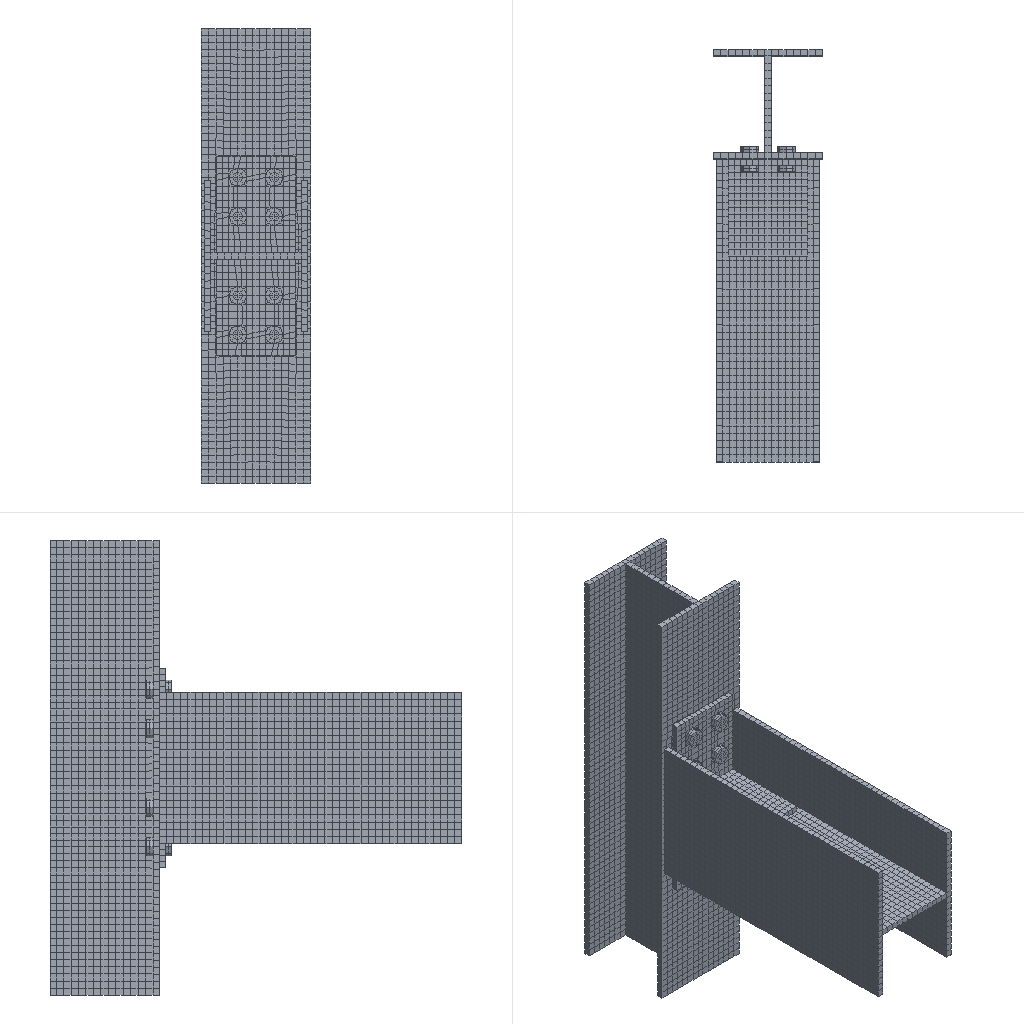Simulation study | abaqus
Set-up summary:
category,name,step,type,value,unit,region
solver,abaqus
solver,version,,,Abaqus/Standard 2020
units,not stated in the deck,,not stated
analysis,deck,,coupled temperature-displacement,coupled temperature-displacement
load_step,Step-1,Step-1,coupled temperature-displacement
load_step,requested,,,1
mesh,nodes,,,14096
mesh,elements,,,6914
element_type,C3D8T,,solid,2838
element_type,C3D8RT,,solid,4076
load,load commands in deck,,count,1
bc,support commands in deck,,count,2
material,STEEL,,in results
material,TIMBER,,in results
check,setup vs results,,match,"per instance, exact: element labels, types and connectivity; labels of the nodes the elements use; coordinates not compared"
Abaqus input file, long lists of numbers shortened, first 390 of 3058 lines:
*Heading
** Job name: Job-2 Model name: Model-11
** Generated by: Abaqus/CAE 2020
*Preprint, echo=NO, model=NO, history=NO, contact=NO
**
** PARTS
**
*Part, name=beam-jiedian
*Node
      1,          10.,         120.,           0.
      2,          10.,           0.,           0.
** (4814 more lines like these left out)
*Element, type=C3D8RT
   1,   25,   18,   17,   26,  137,  130,  129,  138
   2,   16,   27,   26,   17,  128,  139,  138,  129
** (2308 more lines like these left out)
*Nset, nset=Set-5, generate
    1,  4816,     1
*Elset, elset=Set-5, generate
    1,  2310,     1
** Section: timber
*Solid Section, elset=Set-5, material=timber
,
*End Part
**
*Part, name=bolt-200
*Node
      1,           8.,         200.,           0.
      2,           0.,         200.,           0.
** (199 more lines like these left out)
*Element, type=C3D8RT
1, 128,  44, 127, 186,  42,   1,  43, 126
2, 127,  46, 129, 186,  43,   2,  45, 126
** (126 more lines like these left out)
*Nset, nset=Set-1, generate
   1,  201,    1
*Elset, elset=Set-1, generate
   1,  128,    1
** Section: steel
*Solid Section, elset=Set-1, material=steel
,
*End Part
**
*Part, name=col-final
*Node
      1,         243.,         170.,         245.
      2,         243.,          10.,         245.
** (5942 more lines like these left out)
*Element, type=C3D8T
  1,  256, 2085,  193,    1,  269, 2325,  268,    6
  2, 2085, 2086,  194,  193, 2325, 2326,  267,  268
** (2836 more lines like these left out)
*Nset, nset=Set-3, generate
    1,  5944,     1
*Elset, elset=Set-3, generate
    1,  2838,     1
** Section: timber
*Solid Section, elset=Set-3, material=timber
,
*End Part
**
*Part, name=steel
*Node
      1,          10.,          75.,         130.
      2,          20.,          75.,         130.
** (862 more lines like these left out)
*Element, type=C3D8RT
1, 158, 160, 567, 565,   1,   2, 149, 152
2, 565, 567, 568, 566, 152, 149, 150, 151
** (369 more lines like these left out)
*Nset, nset=Set-2
   1,   2,   3,   4,   5,   6,   7,   8,   9,  10,  11,  12,  13,  14,  15,  16
  17,  18,  19,  20,  21,  22,  23,  24,  25,  26,  27,  28,  29,  30,  31,  32
** (29 more lines like these left out)
*Elset, elset=Set-2
   1,   2,   3,   4,   5,   6,   7,   8,   9,  10,  11,  12,  13,  14,  15,  16
  17,  18,  19,  20,  21,  22,  23,  24,  25,  26,  27,  28,  29,  30,  31,  32
** (10 more lines like these left out)
*Nset, nset=Set-6, generate
   1,  864,    1
*Elset, elset=Set-6, generate
   1,  371,    1
** Section: steel
*Solid Section, elset=Set-6, material=steel
,
*End Part
**
**
** ASSEMBLY
**
*Assembly, name=Assembly
**
*Instance, name=beam-jiedian-1, part=beam-jiedian
        323.,        -500.,         250.
        323.,        -500.,         250.,         323., -499.293, 250.707,         180.
*End Instance
**
*Instance, name=steel-1, part=steel
        173.,          10.,         370.
        173.,          10.,         370., 172.423, 10.577, 369.423,         120.
*End Instance
**
*Instance, name=steel-2, part=steel
        303.,          10.,         380.
        303.,          10.,         380., 303.577, 9.423, 379.423,         120.
*End Instance
**
*Instance, name=bolt-200-1-lin-2-2-lin-2-1, part=bolt-200
        268.,        -200.,         310.
*End Instance
**
*Instance, name=bolt-200-1-lin-2-1-lin-2-1, part=bolt-200
        268.,        -200.,         245.
*End Instance
**
*Instance, name=bolt-200-1-lin-1-2-lin-2-1, part=bolt-200
        208.,        -200.,         310.
*End Instance
**
*Instance, name=bolt-200-1-lin-2-1-1, part=bolt-200
        208.,        -200.,         245.
*End Instance
**
*Instance, name=bolt-200-1-lin-2-2-lin-2-1-lin-2-1, part=bolt-200
        268.,        -200.,         505.
*End Instance
**
*Instance, name=bolt-200-1-lin-2-1-lin-2-1-lin-2-1, part=bolt-200
        268.,        -200.,         440.
*End Instance
**
*Instance, name=bolt-200-1-lin-2-1-1-lin-2-1, part=bolt-200
        208.,        -200.,         440.
*End Instance
**
*Instance, name=bolt-200-1-lin-1-2-lin-2-1-lin-2-1, part=bolt-200
        208.,        -200.,         505.
*End Instance
**
*Instance, name=col-final-1, part=col-final
*End Instance
**
*Nset, nset=Set-4, instance=col-final-1
    3,    4,    7,    8,   19,   20,   23,   24,   31,   32,   35,   36,   43,   44,   47,   48
   55,   56,   59,   60,   82,   84,   85,   87,   89,   93,  110,  112,  117,  118,  123,  124
** (9 more lines like these left out)
*Elset, elset=Set-4, instance=col-final-1
  261,  262,  263,  264,  265,  266,  267,  268,  269,  270,  271,  272,  273,  677,  678,  679
  680,  681,  682,  683,  684,  685,  686,  687,  688,  689,  805,  910,  948,  975, 1050, 1051
** (4 more lines like these left out)
*Elset, elset=_CP-1-bolt-200-1-lin-2-2-lin-2-1_S6, internal, instance=bolt-200-1-lin-2-2-lin-2-1
  97,  99, 109, 111, 125, 127
*Elset, elset=_CP-1-bolt-200-1-lin-2-2-lin-2-1_S1, internal, instance=bolt-200-1-lin-2-2-lin-2-1
 123, 124
*Surface, type=ELEMENT, name=CP-1-bolt-200-1-lin-2-2-lin-2-1
_CP-1-bolt-200-1-lin-2-2-lin-2-1_S6, S6
_CP-1-bolt-200-1-lin-2-2-lin-2-1_S1, S1
*Elset, elset=_CP-1-steel-1_S3, internal, instance=steel-1, generate
 263,  265,    1
*Elset, elset=_CP-1-steel-1_S2, internal, instance=steel-1, generate
 81,  89,   1
*Elset, elset=_CP-1-steel-1_S6, internal, instance=steel-1
  96,  97, 113, 114, 221, 222, 223, 224, 225, 226, 227, 228, 229, 230, 231, 232
 233, 234, 235, 236, 237, 238, 239, 240, 241, 242, 243, 244, 245, 246, 247, 248
** (1 more lines like these left out)
*Elset, elset=_CP-1-steel-1_S4, internal, instance=steel-1
  95, 115, 142, 143, 144, 145, 146, 147, 148, 149, 150, 151, 152, 153, 154, 155
 156, 157, 158, 159, 160, 161, 162, 163, 164, 165, 166, 167, 202, 204, 206
*Elset, elset=_CP-1-steel-1_S5, internal, instance=steel-1
 14, 16
*Elset, elset=_CP-1-steel-1_S1, internal, instance=steel-1
  41,  42,  43,  44,  45,  46,  47,  48,  49,  50,  51,  52,  65,  66,  67,  68
  69,  70,  75,  76,  77,  78,  79,  80,  90,  91,  92,  93,  94,  95,  96,  97
** (3 more lines like these left out)
*Surface, type=ELEMENT, name=CP-1-steel-1
_CP-1-steel-1_S3, S3
_CP-1-steel-1_S2, S2
_CP-1-steel-1_S6, S6
_CP-1-steel-1_S4, S4
_CP-1-steel-1_S5, S5
_CP-1-steel-1_S1, S1
*Elset, elset=_CP-2-bolt-200-1-lin-2-2-lin-2-1_S5, internal, instance=bolt-200-1-lin-2-2-lin-2-1
  97,  98,  99, 100, 109, 110, 111, 112, 125, 126, 127, 128
*Elset, elset=_CP-2-bolt-200-1-lin-2-2-lin-2-1_S6, internal, instance=bolt-200-1-lin-2-2-lin-2-1, generate
 121,  124,    1
*Surface, type=ELEMENT, name=CP-2-bolt-200-1-lin-2-2-lin-2-1
_CP-2-bolt-200-1-lin-2-2-lin-2-1_S5, S5
_CP-2-bolt-200-1-lin-2-2-lin-2-1_S6, S6
*Elset, elset=_CP-2-steel-1_S1, internal, instance=steel-1
  59,  60,  61,  62,  63,  64, 128, 129, 130, 131, 132, 133
*Elset, elset=_CP-2-steel-1_S2, internal, instance=steel-1, generate
 71,  74,   1
*Surface, type=ELEMENT, name=CP-2-steel-1
_CP-2-steel-1_S1, S1
_CP-2-steel-1_S2, S2
*Elset, elset=_CP-3-bolt-200-1-lin-2-2-lin-2-1_S3, internal, instance=bolt-200-1-lin-2-2-lin-2-1
  1,  5,  7, 10, 14, 27, 30, 62, 65, 66
*Elset, elset=_CP-3-bolt-200-1-lin-2-2-lin-2-1_S4, internal, instance=bolt-200-1-lin-2-2-lin-2-1
  3,  6,  9, 13, 25, 29, 63
*Elset, elset=_CP-3-bolt-200-1-lin-2-2-lin-2-1_S2, internal, instance=bolt-200-1-lin-2-2-lin-2-1
 12, 16, 17, 37, 38, 39, 40
*Surface, type=ELEMENT, name=CP-3-bolt-200-1-lin-2-2-lin-2-1
_CP-3-bolt-200-1-lin-2-2-lin-2-1_S3, S3
_CP-3-bolt-200-1-lin-2-2-lin-2-1_S4, S4
_CP-3-bolt-200-1-lin-2-2-lin-2-1_S2, S2
*Elset, elset=_CP-3-steel-1_S6, internal, instance=steel-1
 90, 91, 94, 95
*Elset, elset=_CP-3-steel-1_S4, internal, instance=steel-1
  92,  93,  96,  97,  98,  99, 100
*Surface, type=ELEMENT, name=CP-3-steel-1
_CP-3-steel-1_S6, S6
_CP-3-steel-1_S4, S4
*Elset, elset=_CP-3-steel-2_S1, internal, instance=steel-2
  59,  60,  61,  62,  63,  64, 128, 129, 130, 131, 132, 133
*Elset, elset=_CP-3-steel-2_S2, internal, instance=steel-2, generate
 71,  74,   1
*Surface, type=ELEMENT, name=CP-3-steel-2
_CP-3-steel-2_S1, S1
_CP-3-steel-2_S2, S2
*Elset, elset=_CP-4-bolt-200-1-lin-2-1-lin-2-1_S6, internal, instance=bolt-200-1-lin-2-1-lin-2-1
  97,  99, 109, 111, 125, 127
*Elset, elset=_CP-4-bolt-200-1-lin-2-1-lin-2-1_S1, internal, instance=bolt-200-1-lin-2-1-lin-2-1
 123, 124
*Surface, type=ELEMENT, name=CP-4-bolt-200-1-lin-2-1-lin-2-1
_CP-4-bolt-200-1-lin-2-1-lin-2-1_S6, S6
_CP-4-bolt-200-1-lin-2-1-lin-2-1_S1, S1
*Elset, elset=_CP-4-steel-1_S6, internal, instance=steel-1
 90, 91, 94, 95
*Elset, elset=_CP-4-steel-1_S4, internal, instance=steel-1
  92,  93,  96,  97,  98,  99, 100
*Surface, type=ELEMENT, name=CP-4-steel-1
_CP-4-steel-1_S6, S6
_CP-4-steel-1_S4, S4
*Elset, elset=_CP-5-bolt-200-1-lin-2-1-lin-2-1_S5, internal, instance=bolt-200-1-lin-2-1-lin-2-1
  97,  98,  99, 100, 109, 110, 111, 112, 125, 126, 127, 128
*Elset, elset=_CP-5-bolt-200-1-lin-2-1-lin-2-1_S6, internal, instance=bolt-200-1-lin-2-1-lin-2-1, generate
 121,  124,    1
*Surface, type=ELEMENT, name=CP-5-bolt-200-1-lin-2-1-lin-2-1
_CP-5-bolt-200-1-lin-2-1-lin-2-1_S5, S5
_CP-5-bolt-200-1-lin-2-1-lin-2-1_S6, S6
*Elset, elset=_CP-5-steel-1_S3, internal, instance=steel-1, generate
 263,  265,    1
*Elset, elset=_CP-5-steel-1_S2, internal, instance=steel-1, generate
 81,  89,   1
*Elset, elset=_CP-5-steel-1_S6, internal, instance=steel-1
   7,   8,   9,  10,  11,  12,  96,  97, 113, 114, 221, 222, 223, 224, 225, 226
 227, 228, 229, 230, 231, 232, 233, 234, 235, 236, 237, 238, 239, 240, 241, 242
** (2 more lines like these left out)
*Elset, elset=_CP-5-steel-1_S4, internal, instance=steel-1
  95, 115, 142, 143, 144, 145, 146, 147, 148, 149, 150, 151, 152, 153, 154, 155
 156, 157, 158, 159, 160, 161, 162, 163, 164, 165, 166, 167, 202, 204, 206
*Elset, elset=_CP-5-steel-1_S5, internal, instance=steel-1
 14, 16
*Elset, elset=_CP-5-steel-1_S1, internal, instance=steel-1
  41,  42,  43,  44,  45,  46,  47,  48,  49,  50,  51,  52,  65,  66,  67,  68
  69,  70,  75,  76,  77,  78,  79,  80,  90,  91,  92,  93,  94,  95,  96,  97
** (3 more lines like these left out)
*Surface, type=ELEMENT, name=CP-5-steel-1
_CP-5-steel-1_S3, S3
_CP-5-steel-1_S2, S2
_CP-5-steel-1_S6, S6
_CP-5-steel-1_S4, S4
_CP-5-steel-1_S5, S5
_CP-5-steel-1_S1, S1
*Elset, elset=_CP-6-bolt-200-1-lin-2-1-lin-2-1_S3, internal, instance=bolt-200-1-lin-2-1-lin-2-1
  1,  5,  7, 10, 14, 27, 30, 62, 65, 66
*Elset, elset=_CP-6-bolt-200-1-lin-2-1-lin-2-1_S4, internal, instance=bolt-200-1-lin-2-1-lin-2-1
  3,  6,  9, 13, 25, 29, 63
*Elset, elset=_CP-6-bolt-200-1-lin-2-1-lin-2-1_S2, internal, instance=bolt-200-1-lin-2-1-lin-2-1
 12, 16, 17, 37, 38, 39, 40
*Surface, type=ELEMENT, name=CP-6-bolt-200-1-lin-2-1-lin-2-1
_CP-6-bolt-200-1-lin-2-1-lin-2-1_S3, S3
_CP-6-bolt-200-1-lin-2-1-lin-2-1_S4, S4
_CP-6-bolt-200-1-lin-2-1-lin-2-1_S2, S2
*Elset, elset=_CP-6-steel-1_S6, internal, instance=steel-1
 110, 111, 112, 115, 118
*Elset, elset=_CP-6-steel-1_S4, internal, instance=steel-1
 113, 114, 116, 117, 119, 120, 121
*Surface, type=ELEMENT, name=CP-6-steel-1
_CP-6-steel-1_S6, S6
_CP-6-steel-1_S4, S4
*Elset, elset=_CP-7-bolt-200-1-lin-1-2-lin-2-1_S6, internal, instance=bolt-200-1-lin-1-2-lin-2-1
  97,  99, 109, 111, 125, 127
*Elset, elset=_CP-7-bolt-200-1-lin-1-2-lin-2-1_S1, internal, instance=bolt-200-1-lin-1-2-lin-2-1
 123, 124
*Surface, type=ELEMENT, name=CP-7-bolt-200-1-lin-1-2-lin-2-1
_CP-7-bolt-200-1-lin-1-2-lin-2-1_S6, S6
_CP-7-bolt-200-1-lin-1-2-lin-2-1_S1, S1
*Elset, elset=_CP-7-steel-1_S6, internal, instance=steel-1
 110, 111, 112, 115, 118
*Elset, elset=_CP-7-steel-1_S4, internal, instance=steel-1
 113, 114, 116, 117, 119, 120, 121
*Surface, type=ELEMENT, name=CP-7-steel-1
_CP-7-steel-1_S6, S6
_CP-7-steel-1_S4, S4
*Elset, elset=_CP-8-bolt-200-1-lin-1-2-lin-2-1_S5, internal, instance=bolt-200-1-lin-1-2-lin-2-1
  97,  98,  99, 100, 109, 110, 111, 112, 125, 126, 127, 128
*Elset, elset=_CP-8-bolt-200-1-lin-1-2-lin-2-1_S6, internal, instance=bolt-200-1-lin-1-2-lin-2-1, generate
 121,  124,    1
*Surface, type=ELEMENT, name=CP-8-bolt-200-1-lin-1-2-lin-2-1
_CP-8-bolt-200-1-lin-1-2-lin-2-1_S5, S5
_CP-8-bolt-200-1-lin-1-2-lin-2-1_S6, S6
*Elset, elset=_CP-8-steel-1_S3, internal, instance=steel-1, generate
 263,  265,    1
*Elset, elset=_CP-8-steel-1_S6, internal, instance=steel-1
  71,  73,  96,  97, 221, 222, 223, 224, 225, 226, 227, 228, 229, 230, 231, 232
 233, 234, 235, 236, 237, 238, 239, 240, 241, 242, 243, 244, 245, 246, 247, 248
** (1 more lines like these left out)
*Elset, elset=_CP-8-steel-1_S2, internal, instance=steel-1, generate
 81,  89,   1
*Elset, elset=_CP-8-steel-1_S4, internal, instance=steel-1
  95, 142, 143, 144, 145, 146, 147, 148, 149, 150, 151, 152, 153, 154, 155, 156
 157, 158, 159, 160, 161, 162, 163, 164, 165, 166, 167, 202, 204, 206
*Elset, elset=_CP-8-steel-1_S5, internal, instance=steel-1
 14, 16
*Elset, elset=_CP-8-steel-1_S1, internal, instance=steel-1
  41,  42,  43,  44,  45,  46,  47,  48,  49,  50,  51,  52,  65,  66,  67,  68
  69,  70,  75,  76,  77,  78,  79,  80,  90,  91,  92,  93,  94,  95,  96,  97
** (3 more lines like these left out)
*Surface, type=ELEMENT, name=CP-8-steel-1
_CP-8-steel-1_S3, S3
_CP-8-steel-1_S6, S6
_CP-8-steel-1_S2, S2
_CP-8-steel-1_S4, S4
_CP-8-steel-1_S5, S5
_CP-8-steel-1_S1, S1
*Elset, elset=_CP-9-bolt-200-1-lin-1-2-lin-2-1_S3, internal, instance=bolt-200-1-lin-1-2-lin-2-1
  1,  5,  7, 10, 14, 27, 30, 62, 65, 66
*Elset, elset=_CP-9-bolt-200-1-lin-1-2-lin-2-1_S4, internal, instance=bolt-200-1-lin-1-2-lin-2-1
  3,  6,  9, 13, 25, 29, 63
*Elset, elset=_CP-9-bolt-200-1-lin-1-2-lin-2-1_S2, internal, instance=bolt-200-1-lin-1-2-lin-2-1
 12, 16, 17, 37, 38, 39, 40
*Surface, type=ELEMENT, name=CP-9-bolt-200-1-lin-1-2-lin-2-1
_CP-9-bolt-200-1-lin-1-2-lin-2-1_S3, S3
_CP-9-bolt-200-1-lin-1-2-lin-2-1_S4, S4
_CP-9-bolt-200-1-lin-1-2-lin-2-1_S2, S2
*Elset, elset=_CP-9-steel-1_S4, internal, instance=steel-1
 207, 208, 209, 210, 212, 213
*Elset, elset=_CP-9-steel-1_S6, internal, instance=steel-1
 211, 214, 215, 216, 217
*Surface, type=ELEMENT, name=CP-9-steel-1
_CP-9-steel-1_S4, S4
_CP-9-steel-1_S6, S6
*Elset, elset=_CP-10-bolt-200-1-lin-2-1-1_S6, internal, instance=bolt-200-1-lin-2-1-1
  97,  99, 109, 111, 125, 127
*Elset, elset=_CP-10-bolt-200-1-lin-2-1-1_S1, internal, instance=bolt-200-1-lin-2-1-1
 123, 124
*Surface, type=ELEMENT, name=CP-10-bolt-200-1-lin-2-1-1
_CP-10-bolt-200-1-lin-2-1-1_S6, S6
_CP-10-bolt-200-1-lin-2-1-1_S1, S1
*Elset, elset=_CP-10-steel-1_S4, internal, instance=steel-1
  13,  14,  15,  16, 123, 125, 127, 211, 215, 305, 306
*Elset, elset=_CP-10-steel-1_S5, internal, instance=steel-1
   9,  12, 134, 135, 263, 264, 265, 305, 306
*Elset, elset=_CP-10-steel-1_S2, internal, instance=steel-1
  90,  91,  92,  93,  94,  95,  96,  97,  98,  99, 100, 101, 102, 103, 104, 105
 106, 107, 108, 109, 122, 123, 124, 125, 126, 127, 207, 208, 209, 210, 211, 212
** (1 more lines like these left out)
*Elset, elset=_CP-10-steel-1_S6, internal, instance=steel-1
   1,   2,   3,   4,   5,   6, 122, 124, 126, 209, 210, 212, 213
*Elset, elset=_CP-10-steel-1_S3, internal, instance=steel-1
 138, 139, 180, 181, 182, 198, 199, 200
*Elset, elset=_CP-10-steel-1_S1, internal, instance=steel-1
  17,  18,  19,  20,  21,  22,  23,  24,  25,  26,  27,  28,  29,  30,  31, 122
 123, 124, 125, 126, 127, 201, 202, 203, 204, 205, 206
*Surface, type=ELEMENT, name=CP-10-steel-1
_CP-10-steel-1_S4, S4
_CP-10-steel-1_S5, S5
_CP-10-steel-1_S2, S2
_CP-10-steel-1_S6, S6
_CP-10-steel-1_S3, S3
_CP-10-steel-1_S1, S1
*Elset, elset=_CP-11-bolt-200-1-lin-2-1-1_S5, internal, instance=bolt-200-1-lin-2-1-1
  97,  98,  99, 100, 109, 110, 111, 112, 125, 126, 127, 128
*Elset, elset=_CP-11-bolt-200-1-lin-2-1-1_S6, internal, instance=bolt-200-1-lin-2-1-1, generate
 121,  124,    1
*Surface, type=ELEMENT, name=CP-11-bolt-200-1-lin-2-1-1
_CP-11-bolt-200-1-lin-2-1-1_S5, S5
_CP-11-bolt-200-1-lin-2-1-1_S6, S6
*Elset, elset=_CP-11-steel-1_S4, internal, instance=steel-1
 207, 208, 209, 210, 212, 213
*Elset, elset=_CP-11-steel-1_S6, internal, instance=steel-1
 211, 214, 215, 216, 217
*Surface, type=ELEMENT, name=CP-11-steel-1
_CP-11-steel-1_S4, S4
_CP-11-steel-1_S6, S6
*Elset, elset=_CP-11-steel-2_S4, internal, instance=steel-2
  13,  14,  15,  16, 123, 125, 127, 211, 215, 305, 306
*Elset, elset=_CP-11-steel-2_S5, internal, instance=steel-2
   9,  12, 134, 135, 263, 264, 265, 305, 306
Last 668 lines:
 101,  104,    1
*Surface, type=ELEMENT, name=_Int-1_gcs0_797, internal
__Int-1_gcs0_797_S5, S5
*Elset, elset=__Int-1_gcs0_799_S3, internal, instance=bolt-200-1-lin-2-2-lin-2-1-lin-2-1
 1, 5
*Elset, elset=__Int-1_gcs0_799_S4, internal, instance=bolt-200-1-lin-2-2-lin-2-1-lin-2-1
 3, 6
*Surface, type=ELEMENT, name=_Int-1_gcs0_799, internal
__Int-1_gcs0_799_S3, S3
__Int-1_gcs0_799_S4, S4
*Elset, elset=__Int-1_gcs0_801_S5, internal, instance=bolt-200-1-lin-2-2-lin-2-1-lin-2-1, generate
 109,  112,    1
*Surface, type=ELEMENT, name=_Int-1_gcs0_801, internal
__Int-1_gcs0_801_S5, S5
*Elset, elset=__Int-1_gcs0_807_S3, internal, instance=bolt-200-1-lin-2-1-lin-2-1-lin-2-1
 62, 65, 66
*Elset, elset=__Int-1_gcs0_807_S4, internal, instance=bolt-200-1-lin-2-1-lin-2-1-lin-2-1
 63,
*Surface, type=ELEMENT, name=_Int-1_gcs0_807, internal
__Int-1_gcs0_807_S3, S3
__Int-1_gcs0_807_S4, S4
*Elset, elset=__Int-1_gcs0_808_S3, internal, instance=bolt-200-1-lin-2-1-lin-2-1-lin-2-1
 31,
*Elset, elset=__Int-1_gcs0_808_S4, internal, instance=bolt-200-1-lin-2-1-lin-2-1-lin-2-1
 32,
*Elset, elset=__Int-1_gcs0_808_S2, internal, instance=bolt-200-1-lin-2-1-lin-2-1-lin-2-1
 34, 35
*Surface, type=ELEMENT, name=_Int-1_gcs0_808, internal
__Int-1_gcs0_808_S3, S3
__Int-1_gcs0_808_S4, S4
__Int-1_gcs0_808_S2, S2
*Elset, elset=__Int-1_gcs0_810_S3, internal, instance=bolt-200-1-lin-2-1-lin-2-1-lin-2-1
  7, 10
*Elset, elset=__Int-1_gcs0_810_S4, internal, instance=bolt-200-1-lin-2-1-lin-2-1-lin-2-1
 9,
*Elset, elset=__Int-1_gcs0_810_S2, internal, instance=bolt-200-1-lin-2-1-lin-2-1-lin-2-1
 12,
*Surface, type=ELEMENT, name=_Int-1_gcs0_810, internal
__Int-1_gcs0_810_S3, S3
__Int-1_gcs0_810_S4, S4
__Int-1_gcs0_810_S2, S2
*Elset, elset=__Int-1_gcs0_812_S4, internal, instance=bolt-200-1-lin-2-1-lin-2-1-lin-2-1
 19, 22
*Elset, elset=__Int-1_gcs0_812_S3, internal, instance=bolt-200-1-lin-2-1-lin-2-1-lin-2-1
 21,
*Elset, elset=__Int-1_gcs0_812_S2, internal, instance=bolt-200-1-lin-2-1-lin-2-1-lin-2-1
 24,
*Surface, type=ELEMENT, name=_Int-1_gcs0_812, internal
__Int-1_gcs0_812_S4, S4
__Int-1_gcs0_812_S3, S3
__Int-1_gcs0_812_S2, S2
*Elset, elset=__Int-1_gcs0_837_S5, internal, instance=bolt-200-1-lin-2-1-lin-2-1-lin-2-1, generate
  97,  100,    1
*Surface, type=ELEMENT, name=_Int-1_gcs0_837, internal
__Int-1_gcs0_837_S5, S5
*Elset, elset=__Int-1_gcs0_839_S5, internal, instance=bolt-200-1-lin-2-1-lin-2-1-lin-2-1, generate
 113,  116,    1
*Surface, type=ELEMENT, name=_Int-1_gcs0_839, internal
__Int-1_gcs0_839_S5, S5
*Elset, elset=__Int-1_gcs0_842_S4, internal, instance=bolt-200-1-lin-2-1-lin-2-1-lin-2-1
 13,
*Elset, elset=__Int-1_gcs0_842_S3, internal, instance=bolt-200-1-lin-2-1-lin-2-1-lin-2-1
 14,
*Elset, elset=__Int-1_gcs0_842_S2, internal, instance=bolt-200-1-lin-2-1-lin-2-1-lin-2-1
 16, 17
*Surface, type=ELEMENT, name=_Int-1_gcs0_842, internal
__Int-1_gcs0_842_S4, S4
__Int-1_gcs0_842_S3, S3
__Int-1_gcs0_842_S2, S2
*Elset, elset=__Int-1_gcs0_845_S5, internal, instance=bolt-200-1-lin-2-1-lin-2-1-lin-2-1, generate
 125,  128,    1
*Surface, type=ELEMENT, name=_Int-1_gcs0_845, internal
__Int-1_gcs0_845_S5, S5
*Elset, elset=__Int-1_gcs0_854_S4, internal, instance=bolt-200-1-lin-2-1-lin-2-1-lin-2-1
 25, 29
*Elset, elset=__Int-1_gcs0_854_S3, internal, instance=bolt-200-1-lin-2-1-lin-2-1-lin-2-1
 27, 30
*Surface, type=ELEMENT, name=_Int-1_gcs0_854, internal
__Int-1_gcs0_854_S4, S4
__Int-1_gcs0_854_S3, S3
*Elset, elset=__Int-1_gcs0_859_S3, internal, instance=bolt-200-1-lin-2-1-lin-2-1-lin-2-1, generate
 105,  108,    1
*Surface, type=ELEMENT, name=_Int-1_gcs0_859, internal
__Int-1_gcs0_859_S3, S3
*Elset, elset=__Int-1_gcs0_865_S6, internal, instance=bolt-200-1-lin-2-1-lin-2-1-lin-2-1, generate
 121,  124,    1
*Surface, type=ELEMENT, name=_Int-1_gcs0_865, internal
__Int-1_gcs0_865_S6, S6
*Elset, elset=__Int-1_gcs0_869_S2, internal, instance=bolt-200-1-lin-2-1-lin-2-1-lin-2-1, generate
 37,  40,   1
*Surface, type=ELEMENT, name=_Int-1_gcs0_869, internal
__Int-1_gcs0_869_S2, S2
*Elset, elset=__Int-1_gcs0_871_S3, internal, instance=bolt-200-1-lin-2-1-lin-2-1-lin-2-1, generate
 117,  120,    1
*Surface, type=ELEMENT, name=_Int-1_gcs0_871, internal
__Int-1_gcs0_871_S3, S3
*Elset, elset=__Int-1_gcs0_881_S5, internal, instance=bolt-200-1-lin-2-1-lin-2-1-lin-2-1, generate
 101,  104,    1
*Surface, type=ELEMENT, name=_Int-1_gcs0_881, internal
__Int-1_gcs0_881_S5, S5
*Elset, elset=__Int-1_gcs0_883_S3, internal, instance=bolt-200-1-lin-2-1-lin-2-1-lin-2-1
 1, 5
*Elset, elset=__Int-1_gcs0_883_S4, internal, instance=bolt-200-1-lin-2-1-lin-2-1-lin-2-1
 3, 6
*Surface, type=ELEMENT, name=_Int-1_gcs0_883, internal
__Int-1_gcs0_883_S3, S3
__Int-1_gcs0_883_S4, S4
*Elset, elset=__Int-1_gcs0_885_S5, internal, instance=bolt-200-1-lin-2-1-lin-2-1-lin-2-1, generate
 109,  112,    1
*Surface, type=ELEMENT, name=_Int-1_gcs0_885, internal
__Int-1_gcs0_885_S5, S5
*Elset, elset=__Int-1_gcs0_891_S3, internal, instance=bolt-200-1-lin-2-1-1-lin-2-1
 62, 65, 66
*Elset, elset=__Int-1_gcs0_891_S4, internal, instance=bolt-200-1-lin-2-1-1-lin-2-1
 63,
*Surface, type=ELEMENT, name=_Int-1_gcs0_891, internal
__Int-1_gcs0_891_S3, S3
__Int-1_gcs0_891_S4, S4
*Elset, elset=__Int-1_gcs0_892_S3, internal, instance=bolt-200-1-lin-2-1-1-lin-2-1
 31,
*Elset, elset=__Int-1_gcs0_892_S4, internal, instance=bolt-200-1-lin-2-1-1-lin-2-1
 32,
*Elset, elset=__Int-1_gcs0_892_S2, internal, instance=bolt-200-1-lin-2-1-1-lin-2-1
 34, 35
*Surface, type=ELEMENT, name=_Int-1_gcs0_892, internal
__Int-1_gcs0_892_S3, S3
__Int-1_gcs0_892_S4, S4
__Int-1_gcs0_892_S2, S2
*Elset, elset=__Int-1_gcs0_894_S3, internal, instance=bolt-200-1-lin-2-1-1-lin-2-1
  7, 10
*Elset, elset=__Int-1_gcs0_894_S4, internal, instance=bolt-200-1-lin-2-1-1-lin-2-1
 9,
*Elset, elset=__Int-1_gcs0_894_S2, internal, instance=bolt-200-1-lin-2-1-1-lin-2-1
 12,
*Surface, type=ELEMENT, name=_Int-1_gcs0_894, internal
__Int-1_gcs0_894_S3, S3
__Int-1_gcs0_894_S4, S4
__Int-1_gcs0_894_S2, S2
*Elset, elset=__Int-1_gcs0_896_S4, internal, instance=bolt-200-1-lin-2-1-1-lin-2-1
 19, 22
*Elset, elset=__Int-1_gcs0_896_S3, internal, instance=bolt-200-1-lin-2-1-1-lin-2-1
 21,
*Elset, elset=__Int-1_gcs0_896_S2, internal, instance=bolt-200-1-lin-2-1-1-lin-2-1
 24,
*Surface, type=ELEMENT, name=_Int-1_gcs0_896, internal
__Int-1_gcs0_896_S4, S4
__Int-1_gcs0_896_S3, S3
__Int-1_gcs0_896_S2, S2
*Elset, elset=__Int-1_gcs0_921_S5, internal, instance=bolt-200-1-lin-2-1-1-lin-2-1, generate
  97,  100,    1
*Surface, type=ELEMENT, name=_Int-1_gcs0_921, internal
__Int-1_gcs0_921_S5, S5
*Elset, elset=__Int-1_gcs0_923_S5, internal, instance=bolt-200-1-lin-2-1-1-lin-2-1, generate
 113,  116,    1
*Surface, type=ELEMENT, name=_Int-1_gcs0_923, internal
__Int-1_gcs0_923_S5, S5
*Elset, elset=__Int-1_gcs0_926_S4, internal, instance=bolt-200-1-lin-2-1-1-lin-2-1
 13,
*Elset, elset=__Int-1_gcs0_926_S3, internal, instance=bolt-200-1-lin-2-1-1-lin-2-1
 14,
*Elset, elset=__Int-1_gcs0_926_S2, internal, instance=bolt-200-1-lin-2-1-1-lin-2-1
 16, 17
*Surface, type=ELEMENT, name=_Int-1_gcs0_926, internal
__Int-1_gcs0_926_S4, S4
__Int-1_gcs0_926_S3, S3
__Int-1_gcs0_926_S2, S2
*Elset, elset=__Int-1_gcs0_929_S5, internal, instance=bolt-200-1-lin-2-1-1-lin-2-1, generate
 125,  128,    1
*Surface, type=ELEMENT, name=_Int-1_gcs0_929, internal
__Int-1_gcs0_929_S5, S5
*Elset, elset=__Int-1_gcs0_938_S4, internal, instance=bolt-200-1-lin-2-1-1-lin-2-1
 25, 29
*Elset, elset=__Int-1_gcs0_938_S3, internal, instance=bolt-200-1-lin-2-1-1-lin-2-1
 27, 30
*Surface, type=ELEMENT, name=_Int-1_gcs0_938, internal
__Int-1_gcs0_938_S4, S4
__Int-1_gcs0_938_S3, S3
*Elset, elset=__Int-1_gcs0_943_S3, internal, instance=bolt-200-1-lin-2-1-1-lin-2-1, generate
 105,  108,    1
*Surface, type=ELEMENT, name=_Int-1_gcs0_943, internal
__Int-1_gcs0_943_S3, S3
*Elset, elset=__Int-1_gcs0_949_S6, internal, instance=bolt-200-1-lin-2-1-1-lin-2-1, generate
 121,  124,    1
*Surface, type=ELEMENT, name=_Int-1_gcs0_949, internal
__Int-1_gcs0_949_S6, S6
*Elset, elset=__Int-1_gcs0_953_S2, internal, instance=bolt-200-1-lin-2-1-1-lin-2-1, generate
 37,  40,   1
*Surface, type=ELEMENT, name=_Int-1_gcs0_953, internal
__Int-1_gcs0_953_S2, S2
*Elset, elset=__Int-1_gcs0_955_S3, internal, instance=bolt-200-1-lin-2-1-1-lin-2-1, generate
 117,  120,    1
*Surface, type=ELEMENT, name=_Int-1_gcs0_955, internal
__Int-1_gcs0_955_S3, S3
*Elset, elset=__Int-1_gcs0_965_S5, internal, instance=bolt-200-1-lin-2-1-1-lin-2-1, generate
 101,  104,    1
*Surface, type=ELEMENT, name=_Int-1_gcs0_965, internal
__Int-1_gcs0_965_S5, S5
*Elset, elset=__Int-1_gcs0_967_S3, internal, instance=bolt-200-1-lin-2-1-1-lin-2-1
 1, 5
*Elset, elset=__Int-1_gcs0_967_S4, internal, instance=bolt-200-1-lin-2-1-1-lin-2-1
 3, 6
*Surface, type=ELEMENT, name=_Int-1_gcs0_967, internal
__Int-1_gcs0_967_S3, S3
__Int-1_gcs0_967_S4, S4
*Elset, elset=__Int-1_gcs0_969_S5, internal, instance=bolt-200-1-lin-2-1-1-lin-2-1, generate
 109,  112,    1
*Surface, type=ELEMENT, name=_Int-1_gcs0_969, internal
__Int-1_gcs0_969_S5, S5
*Elset, elset=__Int-1_gcs0_975_S3, internal, instance=bolt-200-1-lin-1-2-lin-2-1-lin-2-1
 62, 65, 66
*Elset, elset=__Int-1_gcs0_975_S4, internal, instance=bolt-200-1-lin-1-2-lin-2-1-lin-2-1
 63,
*Surface, type=ELEMENT, name=_Int-1_gcs0_975, internal
__Int-1_gcs0_975_S3, S3
__Int-1_gcs0_975_S4, S4
*Elset, elset=__Int-1_gcs0_976_S3, internal, instance=bolt-200-1-lin-1-2-lin-2-1-lin-2-1
 31,
*Elset, elset=__Int-1_gcs0_976_S4, internal, instance=bolt-200-1-lin-1-2-lin-2-1-lin-2-1
 32,
*Elset, elset=__Int-1_gcs0_976_S2, internal, instance=bolt-200-1-lin-1-2-lin-2-1-lin-2-1
 34, 35
*Surface, type=ELEMENT, name=_Int-1_gcs0_976, internal
__Int-1_gcs0_976_S3, S3
__Int-1_gcs0_976_S4, S4
__Int-1_gcs0_976_S2, S2
*Elset, elset=__Int-1_gcs0_978_S3, internal, instance=bolt-200-1-lin-1-2-lin-2-1-lin-2-1
  7, 10
*Elset, elset=__Int-1_gcs0_978_S4, internal, instance=bolt-200-1-lin-1-2-lin-2-1-lin-2-1
 9,
*Elset, elset=__Int-1_gcs0_978_S2, internal, instance=bolt-200-1-lin-1-2-lin-2-1-lin-2-1
 12,
*Surface, type=ELEMENT, name=_Int-1_gcs0_978, internal
__Int-1_gcs0_978_S3, S3
__Int-1_gcs0_978_S4, S4
__Int-1_gcs0_978_S2, S2
*Elset, elset=__Int-1_gcs0_980_S4, internal, instance=bolt-200-1-lin-1-2-lin-2-1-lin-2-1
 19, 22
*Elset, elset=__Int-1_gcs0_980_S3, internal, instance=bolt-200-1-lin-1-2-lin-2-1-lin-2-1
 21,
*Elset, elset=__Int-1_gcs0_980_S2, internal, instance=bolt-200-1-lin-1-2-lin-2-1-lin-2-1
 24,
*Surface, type=ELEMENT, name=_Int-1_gcs0_980, internal
__Int-1_gcs0_980_S4, S4
__Int-1_gcs0_980_S3, S3
__Int-1_gcs0_980_S2, S2
*Elset, elset=__Int-1_gcs0_1005_S5, internal, instance=bolt-200-1-lin-1-2-lin-2-1-lin-2-1, generate
  97,  100,    1
*Surface, type=ELEMENT, name=_Int-1_gcs0_1005, internal
__Int-1_gcs0_1005_S5, S5
*Elset, elset=__Int-1_gcs0_1007_S5, internal, instance=bolt-200-1-lin-1-2-lin-2-1-lin-2-1, generate
 113,  116,    1
*Surface, type=ELEMENT, name=_Int-1_gcs0_1007, internal
__Int-1_gcs0_1007_S5, S5
*Elset, elset=__Int-1_gcs0_1010_S4, internal, instance=bolt-200-1-lin-1-2-lin-2-1-lin-2-1
 13,
*Elset, elset=__Int-1_gcs0_1010_S3, internal, instance=bolt-200-1-lin-1-2-lin-2-1-lin-2-1
 14,
*Elset, elset=__Int-1_gcs0_1010_S2, internal, instance=bolt-200-1-lin-1-2-lin-2-1-lin-2-1
 16, 17
*Surface, type=ELEMENT, name=_Int-1_gcs0_1010, internal
__Int-1_gcs0_1010_S4, S4
__Int-1_gcs0_1010_S3, S3
__Int-1_gcs0_1010_S2, S2
*Elset, elset=__Int-1_gcs0_1013_S5, internal, instance=bolt-200-1-lin-1-2-lin-2-1-lin-2-1, generate
 125,  128,    1
*Surface, type=ELEMENT, name=_Int-1_gcs0_1013, internal
__Int-1_gcs0_1013_S5, S5
*Elset, elset=__Int-1_gcs0_1022_S4, internal, instance=bolt-200-1-lin-1-2-lin-2-1-lin-2-1
 25, 29
*Elset, elset=__Int-1_gcs0_1022_S3, internal, instance=bolt-200-1-lin-1-2-lin-2-1-lin-2-1
 27, 30
*Surface, type=ELEMENT, name=_Int-1_gcs0_1022, internal
__Int-1_gcs0_1022_S4, S4
__Int-1_gcs0_1022_S3, S3
*Elset, elset=__Int-1_gcs0_1027_S3, internal, instance=bolt-200-1-lin-1-2-lin-2-1-lin-2-1, generate
 105,  108,    1
*Surface, type=ELEMENT, name=_Int-1_gcs0_1027, internal
__Int-1_gcs0_1027_S3, S3
*Elset, elset=__Int-1_gcs0_1033_S6, internal, instance=bolt-200-1-lin-1-2-lin-2-1-lin-2-1, generate
 121,  124,    1
*Surface, type=ELEMENT, name=_Int-1_gcs0_1033, internal
__Int-1_gcs0_1033_S6, S6
*Elset, elset=__Int-1_gcs0_1037_S2, internal, instance=bolt-200-1-lin-1-2-lin-2-1-lin-2-1, generate
 37,  40,   1
*Surface, type=ELEMENT, name=_Int-1_gcs0_1037, internal
__Int-1_gcs0_1037_S2, S2
*Elset, elset=__Int-1_gcs0_1039_S3, internal, instance=bolt-200-1-lin-1-2-lin-2-1-lin-2-1, generate
 117,  120,    1
*Surface, type=ELEMENT, name=_Int-1_gcs0_1039, internal
__Int-1_gcs0_1039_S3, S3
*Elset, elset=__Int-1_gcs0_1049_S5, internal, instance=bolt-200-1-lin-1-2-lin-2-1-lin-2-1, generate
 101,  104,    1
*Surface, type=ELEMENT, name=_Int-1_gcs0_1049, internal
__Int-1_gcs0_1049_S5, S5
*Elset, elset=__Int-1_gcs0_1051_S3, internal, instance=bolt-200-1-lin-1-2-lin-2-1-lin-2-1
 1, 5
*Elset, elset=__Int-1_gcs0_1051_S4, internal, instance=bolt-200-1-lin-1-2-lin-2-1-lin-2-1
 3, 6
*Surface, type=ELEMENT, name=_Int-1_gcs0_1051, internal
__Int-1_gcs0_1051_S3, S3
__Int-1_gcs0_1051_S4, S4
*Elset, elset=__Int-1_gcs0_1053_S5, internal, instance=bolt-200-1-lin-1-2-lin-2-1-lin-2-1, generate
 109,  112,    1
*Surface, type=ELEMENT, name=_Int-1_gcs0_1053, internal
__Int-1_gcs0_1053_S5, S5
*Elset, elset=__Int-1_gcs0_1147_S4, internal, instance=col-final-1
 1856,
*Elset, elset=__Int-1_gcs0_1147_S5, internal, instance=col-final-1
 1857,
*Surface, type=ELEMENT, name=_Int-1_gcs0_1147, internal
__Int-1_gcs0_1147_S4, S4
__Int-1_gcs0_1147_S5, S5
*Elset, elset=__Int-1_gcs0_1151_S4, internal, instance=col-final-1
 2675,
*Elset, elset=__Int-1_gcs0_1151_S5, internal, instance=col-final-1
 2676,
*Surface, type=ELEMENT, name=_Int-1_gcs0_1151, internal
__Int-1_gcs0_1151_S4, S4
__Int-1_gcs0_1151_S5, S5
*Elset, elset=__Int-1_gcs0_1164_S4, internal, instance=col-final-1
 1162,
*Elset, elset=__Int-1_gcs0_1164_S5, internal, instance=col-final-1
 1163,
*Surface, type=ELEMENT, name=_Int-1_gcs0_1164, internal
__Int-1_gcs0_1164_S4, S4
__Int-1_gcs0_1164_S5, S5
*Elset, elset=__Int-1_gcs0_1169_S4, internal, instance=col-final-1
 1285,
*Elset, elset=__Int-1_gcs0_1169_S5, internal, instance=col-final-1
 1286,
*Surface, type=ELEMENT, name=_Int-1_gcs0_1169, internal
__Int-1_gcs0_1169_S4, S4
__Int-1_gcs0_1169_S5, S5
*Elset, elset=__Int-1_gcs0_1178_S4, internal, instance=col-final-1
 1542,
*Elset, elset=__Int-1_gcs0_1178_S5, internal, instance=col-final-1
 1543,
*Surface, type=ELEMENT, name=_Int-1_gcs0_1178, internal
__Int-1_gcs0_1178_S4, S4
__Int-1_gcs0_1178_S5, S5
*Elset, elset=__Int-1_gcs0_1191_S4, internal, instance=col-final-1
 1155,
*Elset, elset=__Int-1_gcs0_1191_S5, internal, instance=col-final-1
 1156,
*Surface, type=ELEMENT, name=_Int-1_gcs0_1191, internal
__Int-1_gcs0_1191_S4, S4
__Int-1_gcs0_1191_S5, S5
*Elset, elset=__Int-1_gcs0_1196_S4, internal, instance=col-final-1
 1503,
*Elset, elset=__Int-1_gcs0_1196_S5, internal, instance=col-final-1
 1504,
*Surface, type=ELEMENT, name=_Int-1_gcs0_1196, internal
__Int-1_gcs0_1196_S4, S4
__Int-1_gcs0_1196_S5, S5
*Elset, elset=__Int-1_gcs0_1200_S4, internal, instance=col-final-1
 1824,
*Elset, elset=__Int-1_gcs0_1200_S5, internal, instance=col-final-1
 1825,
*Surface, type=ELEMENT, name=_Int-1_gcs0_1200, internal
__Int-1_gcs0_1200_S4, S4
__Int-1_gcs0_1200_S5, S5
*Elset, elset=__Int-1_gcs0_1218_S4, internal, instance=col-final-1
 1141,
*Elset, elset=__Int-1_gcs0_1218_S5, internal, instance=col-final-1
 1142,
*Surface, type=ELEMENT, name=_Int-1_gcs0_1218, internal
__Int-1_gcs0_1218_S4, S4
__Int-1_gcs0_1218_S5, S5
*Elset, elset=__Int-1_gcs0_1223_S4, internal, instance=col-final-1
 1298,
*Elset, elset=__Int-1_gcs0_1223_S5, internal, instance=col-final-1
 1299,
*Surface, type=ELEMENT, name=_Int-1_gcs0_1223, internal
__Int-1_gcs0_1223_S4, S4
__Int-1_gcs0_1223_S5, S5
*Elset, elset=__Int-1_gcs0_1227_S4, internal, instance=col-final-1
 2836,
*Elset, elset=__Int-1_gcs0_1227_S5, internal, instance=col-final-1
 2837,
*Surface, type=ELEMENT, name=_Int-1_gcs0_1227, internal
__Int-1_gcs0_1227_S4, S4
__Int-1_gcs0_1227_S5, S5
*Elset, elset=__Int-1_gcs0_1231_S4, internal, instance=col-final-1
 1955,
*Elset, elset=__Int-1_gcs0_1231_S5, internal, instance=col-final-1
 1956, 1957
*Surface, type=ELEMENT, name=_Int-1_gcs0_1231, internal
__Int-1_gcs0_1231_S4, S4
__Int-1_gcs0_1231_S5, S5
*Elset, elset=__Int-1_gcs0_1240_S4, internal, instance=col-final-1
 2085,
*Elset, elset=__Int-1_gcs0_1240_S5, internal, instance=col-final-1
 2086,
*Surface, type=ELEMENT, name=_Int-1_gcs0_1240, internal
__Int-1_gcs0_1240_S4, S4
__Int-1_gcs0_1240_S5, S5
*Elset, elset=__Int-1_gcs0_1257_S4, internal, instance=col-final-1
 1329,
*Elset, elset=__Int-1_gcs0_1257_S5, internal, instance=col-final-1
 1330,
*Surface, type=ELEMENT, name=_Int-1_gcs0_1257, internal
__Int-1_gcs0_1257_S4, S4
__Int-1_gcs0_1257_S5, S5
*Elset, elset=__Int-1_gcs0_1260_S4, internal, instance=col-final-1
 1117,
*Elset, elset=__Int-1_gcs0_1260_S5, internal, instance=col-final-1
 1118,
*Surface, type=ELEMENT, name=_Int-1_gcs0_1260, internal
__Int-1_gcs0_1260_S4, S4
__Int-1_gcs0_1260_S5, S5
*Elset, elset=__Int-1_gcs0_1262_S4, internal, instance=col-final-1
 2137,
*Elset, elset=__Int-1_gcs0_1262_S5, internal, instance=col-final-1
 2138,
*Surface, type=ELEMENT, name=_Int-1_gcs0_1262, internal
__Int-1_gcs0_1262_S4, S4
__Int-1_gcs0_1262_S5, S5
*Elset, elset=__Int-1_gcs0_1273_S4, internal, instance=col-final-1
 2117,
*Elset, elset=__Int-1_gcs0_1273_S5, internal, instance=col-final-1
 2118,
*Surface, type=ELEMENT, name=_Int-1_gcs0_1273, internal
__Int-1_gcs0_1273_S4, S4
__Int-1_gcs0_1273_S5, S5
*Elset, elset=__Int-1_gcs0_1278_S4, internal, instance=col-final-1
 1242,
*Elset, elset=__Int-1_gcs0_1278_S5, internal, instance=col-final-1
 1243,
*Surface, type=ELEMENT, name=_Int-1_gcs0_1278, internal
__Int-1_gcs0_1278_S4, S4
__Int-1_gcs0_1278_S5, S5
*Elset, elset=__Int-1_gcs0_1280_S4, internal, instance=col-final-1
 1129,
*Elset, elset=__Int-1_gcs0_1280_S5, internal, instance=col-final-1
 1130,
*Surface, type=ELEMENT, name=_Int-1_gcs0_1280, internal
__Int-1_gcs0_1280_S4, S4
__Int-1_gcs0_1280_S5, S5
*Elset, elset=__Int-1_gcs0_1282_S4, internal, instance=col-final-1
 1522,
*Elset, elset=__Int-1_gcs0_1282_S5, internal, instance=col-final-1
 1523,
*Surface, type=ELEMENT, name=_Int-1_gcs0_1282, internal
__Int-1_gcs0_1282_S4, S4
__Int-1_gcs0_1282_S5, S5
*Elset, elset=__Int-1_gcs0_1289_S4, internal, instance=col-final-1
 1316,
*Elset, elset=__Int-1_gcs0_1289_S5, internal, instance=col-final-1
 1317,
*Surface, type=ELEMENT, name=_Int-1_gcs0_1289, internal
__Int-1_gcs0_1289_S4, S4
__Int-1_gcs0_1289_S5, S5
*Elset, elset=__Int-1_gcs0_1290_S4, internal, instance=col-final-1
 1509,
*Elset, elset=__Int-1_gcs0_1290_S5, internal, instance=col-final-1
 1510,
*Surface, type=ELEMENT, name=_Int-1_gcs0_1290, internal
__Int-1_gcs0_1290_S4, S4
__Int-1_gcs0_1290_S5, S5
*Elset, elset=__Int-1_gcs0_1292_S4, internal, instance=col-final-1
 2105,
*Elset, elset=__Int-1_gcs0_1292_S5, internal, instance=col-final-1
 2106,
*Surface, type=ELEMENT, name=_Int-1_gcs0_1292, internal
__Int-1_gcs0_1292_S4, S4
__Int-1_gcs0_1292_S5, S5
*Elset, elset=__Int-1_gcs0_1294_S4, internal, instance=col-final-1
 2814,
*Elset, elset=__Int-1_gcs0_1294_S5, internal, instance=col-final-1
 2815,
*Surface, type=ELEMENT, name=_Int-1_gcs0_1294, internal
__Int-1_gcs0_1294_S4, S4
__Int-1_gcs0_1294_S5, S5
*Elset, elset=__Int-1_gcs0_1301_S4, internal, instance=col-final-1
 1322,
*Elset, elset=__Int-1_gcs0_1301_S5, internal, instance=col-final-1
 1323,
*Surface, type=ELEMENT, name=_Int-1_gcs0_1301, internal
__Int-1_gcs0_1301_S4, S4
__Int-1_gcs0_1301_S5, S5
*Elset, elset=__Int-1_gcs0_1302_S4, internal, instance=col-final-1
 2475,
*Elset, elset=__Int-1_gcs0_1302_S5, internal, instance=col-final-1
 2476,
*Surface, type=ELEMENT, name=_Int-1_gcs0_1302, internal
__Int-1_gcs0_1302_S4, S4
__Int-1_gcs0_1302_S5, S5
*Elset, elset=__Int-1_gcs0_1303_S4, internal, instance=col-final-1
 1308,
*Elset, elset=__Int-1_gcs0_1303_S5, internal, instance=col-final-1
 1309,
*Surface, type=ELEMENT, name=_Int-1_gcs0_1303, internal
__Int-1_gcs0_1303_S4, S4
__Int-1_gcs0_1303_S5, S5
*Elset, elset=__Int-1_gcs0_1304_S4, internal, instance=col-final-1
 2017, 2018
*Elset, elset=__Int-1_gcs0_1304_S5, internal, instance=col-final-1
 2019,
*Surface, type=ELEMENT, name=_Int-1_gcs0_1304, internal
__Int-1_gcs0_1304_S4, S4
__Int-1_gcs0_1304_S5, S5
*Elset, elset=__Int-1_gcs0_1305_S4, internal, instance=col-final-1
 1149,
*Elset, elset=__Int-1_gcs0_1305_S5, internal, instance=col-final-1
 1150,
*Surface, type=ELEMENT, name=_Int-1_gcs0_1305, internal
__Int-1_gcs0_1305_S4, S4
__Int-1_gcs0_1305_S5, S5
*Elset, elset=__Int-1_gcs0_1306_S4, internal, instance=col-final-1
 1844,
*Elset, elset=__Int-1_gcs0_1306_S5, internal, instance=col-final-1
 1845,
*Surface, type=ELEMENT, name=_Int-1_gcs0_1306, internal
__Int-1_gcs0_1306_S4, S4
__Int-1_gcs0_1306_S5, S5
*Elset, elset=__Int-1_gcs0_1307_S4, internal, instance=col-final-1
 1111,
*Elset, elset=__Int-1_gcs0_1307_S5, internal, instance=col-final-1
 1112,
*Surface, type=ELEMENT, name=_Int-1_gcs0_1307, internal
__Int-1_gcs0_1307_S4, S4
__Int-1_gcs0_1307_S5, S5
*Elset, elset=__Int-1_gcs0_1308_S4, internal, instance=col-final-1
 2358,
*Elset, elset=__Int-1_gcs0_1308_S5, internal, instance=col-final-1
 2359,
*Surface, type=ELEMENT, name=_Int-1_gcs0_1308, internal
__Int-1_gcs0_1308_S4, S4
__Int-1_gcs0_1308_S5, S5
*End Assembly
*Amplitude, name=Amp-1
             0.,              0.,              1.,              1.
*Amplitude, name=Amp-2
             0.,              0.,             10.,           1500.
**
** MATERIALS
**
*Material, name=steel
*Conductivity
45.,
*Density
 7.8e-09,
*Elastic
206000., 0.3
*Expansion
 1e-05,
*Plastic
235.,0.
*Specific Heat
 6.7e+08,
*Material, name=timber
*Conductivity
5.,
*Density
 1.1e-09,
*Elastic
16400., 0.3
*Expansion
 1e-06,
*Plastic
22.,0.
*Specific Heat
 8.9e+08,
**
** INTERACTION PROPERTIES
**
*Surface Interaction, name=IntProp-1
1.,
*Friction, slip tolerance=0.005
 0.3,
*Surface Behavior, pressure-overclosure=HARD
*Gap Conductance
10.,  0.
 0., 0.1
**
** PHYSICAL CONSTANTS
**
*Physical Constants, absolute zero=-273., stefan boltzmann=5.67e-08
**
** INTERACTIONS
**
** Interaction: Int-1
*Contact
*Contact Inclusions, ALL EXTERIOR
*Contact Property Assignment
 ,  , IntProp-1
*Surface Property Assignment, property=GEOMETRIC CORRECTION
_Int-1_gcs0_187, Circumferential, 208., 250.96, 310.,  208., 249.96, 310.
_Int-1_gcs0_188, Circumferential, 268., 250.96, 310.,  268., 249.96, 310.
_Int-1_gcs0_189, Circumferential, 208., 250.96, 245.,  208., 249.96, 245.
_Int-1_gcs0_190, Circumferential, 268., 250.96, 245.,  268., 249.96, 245.
_Int-1_gcs0_371, Circumferential, 268., 250.96, 440.,  268., 249.96, 440.
_Int-1_gcs0_372, Circumferential, 208., 250.96, 440.,  208., 249.96, 440.
_Int-1_gcs0_373, Circumferential, 268., 250.96, 505.,  268., 249.96, 505.
_Int-1_gcs0_374, Circumferential, 208., 250.96, 505.,  208., 249.96, 505.
_Int-1_gcs0_387, Circumferential, 268., 0., 310.,  268., -1., 310.
_Int-1_gcs0_388, Circumferential, 268., 0., 310.,  268., -1., 310.
_Int-1_gcs0_390, Circumferential, 268., 0., 310.,  268., -1., 310.
_Int-1_gcs0_392, Circumferential, 268., 0., 310.,  268., -1., 310.
_Int-1_gcs0_417, Circumferential, 268., -15., 310.,  268., -16., 310.
_Int-1_gcs0_419, Circumferential, 268., 15., 310.,  268., 14., 310.
_Int-1_gcs0_422, Circumferential, 268., 0., 310.,  268., -1., 310.
_Int-1_gcs0_425, Circumferential, 268., -15., 310.,  268., -16., 310.
_Int-1_gcs0_434, Circumferential, 268., 0., 310.,  268., -1., 310.
_Int-1_gcs0_439, Circumferential, 268., 15., 310.,  268., 14., 310.
_Int-1_gcs0_445, Circumferential, 268., -15., 310.,  268., -16., 310.
_Int-1_gcs0_449, Circumferential, 268., 0., 310.,  268., -1., 310.
_Int-1_gcs0_451, Circumferential, 268., 15., 310.,  268., 14., 310.
_Int-1_gcs0_461, Circumferential, 268., 15., 310.,  268., 14., 310.
_Int-1_gcs0_463, Circumferential, 268., 0., 310.,  268., -1., 310.
_Int-1_gcs0_465, Circumferential, 268., -15., 310.,  268., -16., 310.
_Int-1_gcs0_471, Circumferential, 268., 0., 245.,  268., -1., 245.
_Int-1_gcs0_472, Circumferential, 268., 0., 245.,  268., -1., 245.
_Int-1_gcs0_474, Circumferential, 268., 0., 245.,  268., -1., 245.
_Int-1_gcs0_476, Circumferential, 268., 0., 245.,  268., -1., 245.
_Int-1_gcs0_501, Circumferential, 268., -15., 245.,  268., -16., 245.
_Int-1_gcs0_503, Circumferential, 268., 15., 245.,  268., 14., 245.
_Int-1_gcs0_506, Circumferential, 268., 0., 245.,  268., -1., 245.
_Int-1_gcs0_509, Circumferential, 268., -15., 245.,  268., -16., 245.
_Int-1_gcs0_518, Circumferential, 268., 0., 245.,  268., -1., 245.
_Int-1_gcs0_523, Circumferential, 268., 15., 245.,  268., 14., 245.
_Int-1_gcs0_529, Circumferential, 268., -15., 245.,  268., -16., 245.
_Int-1_gcs0_533, Circumferential, 268., 0., 245.,  268., -1., 245.
_Int-1_gcs0_535, Circumferential, 268., 15., 245.,  268., 14., 245.
_Int-1_gcs0_545, Circumferential, 268., 15., 245.,  268., 14., 245.
_Int-1_gcs0_547, Circumferential, 268., 0., 245.,  268., -1., 245.
_Int-1_gcs0_549, Circumferential, 268., -15., 245.,  268., -16., 245.
** (128 more lines like these left out)
** ----------------------------------------------------------------
**
** STEP: Step-1
**
*Step, name=Step-1, nlgeom=YES, inc=1000
*Coupled Temperature-displacement, creep=none, deltmx=1e+13, stabilize=0.0002, allsdtol=0.05, continue=NO
1., 100., 1e-05, 5.
**
** BOUNDARY CONDITIONS
**
** Name: BC-1 Type: 对称/反对称/完全固定
*Boundary
Set-4, ENCASTRE
**
** INTERACTIONS
**
** Interaction: Int-2
*Sradiate, amplitude=Amp-2
Surf-312, R, 1., 1.
**
** OUTPUT REQUESTS
**
*Restart, write, frequency=0
**
** FIELD OUTPUT: F-Output-1
**
*Output, field
*Node Output
CF, NT, RF, RM, RT, U, V
*Element Output, directions=YES
E, HFL, LE, MISES, MISESMAX, NE, PE, PEEQ, PEEQMAX, PEEQT, PEMAG, S, TEMP
*Contact Output
CDISP, CSTRESS
*Radiation Output
FTEMP,
**
** HISTORY OUTPUT: H-Output-1
**
*Output, history, variable=PRESELECT
*End Step
Results summary:
result,step,,partial,increments=2 time=2.0/100.0
result,analysis,,,"coupled temperature-displacement, steady state"
result,last_loadstep,,,1
result,primary field,,,"U, NT11"
result,reaction total,,FX,-0.1425,model units
result,reaction total,,FY,-2572.564,model units
result,reaction total,,FZ,-0.6514,model units